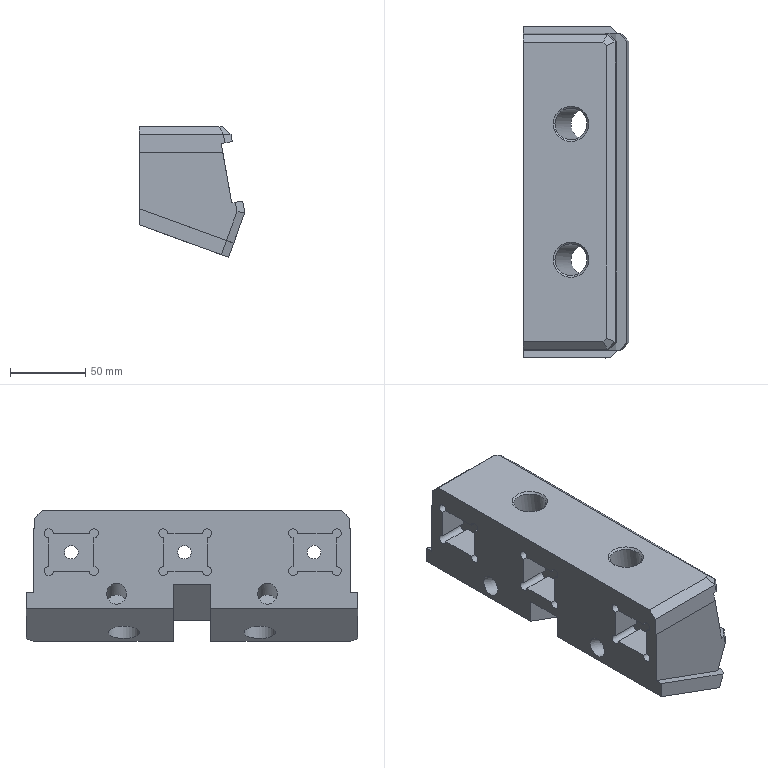Part | STEP file | P011002S002-000 | 1 solid | 358 faces | box 70.019 x 220 x 86.547 mm | volume 835279 mm3 | plane 230 | cylinder 46 | cone 40 | other 40 | spline 2 | commonest cylinder face diameters 6 x12 4.167 x8 4.983 x8 5 x8 9 x3 14 x3